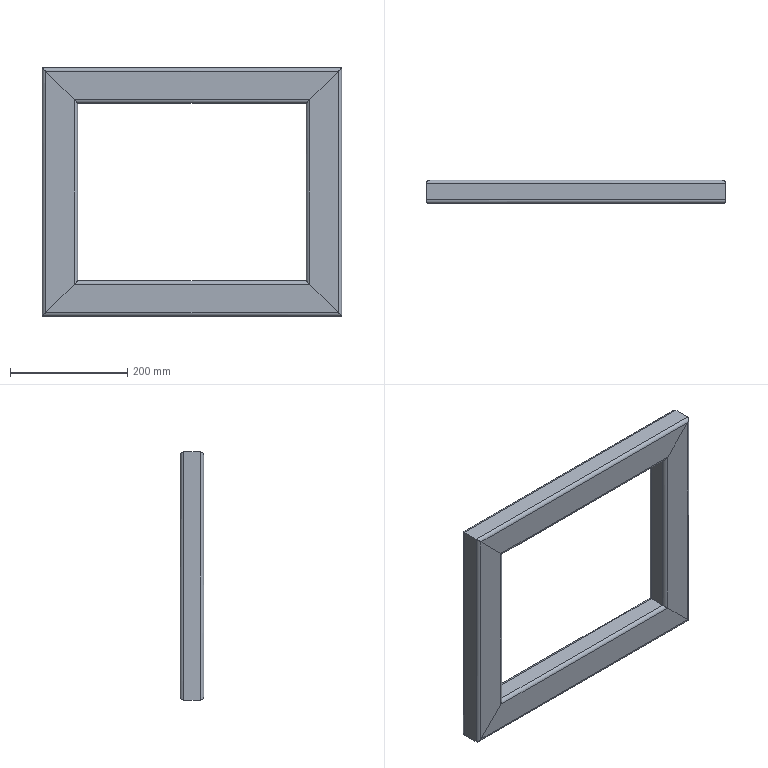Part | SolidWorks | features WeldMemberFeat 1, WeldmentFeature 1 | 4 solids | 72 faces | box 510 x 40 x 423 mm | volume 879378 mm3 | plane 40 | cylinder 32 | commonest cylinder face diameters 6 x16 12 x16